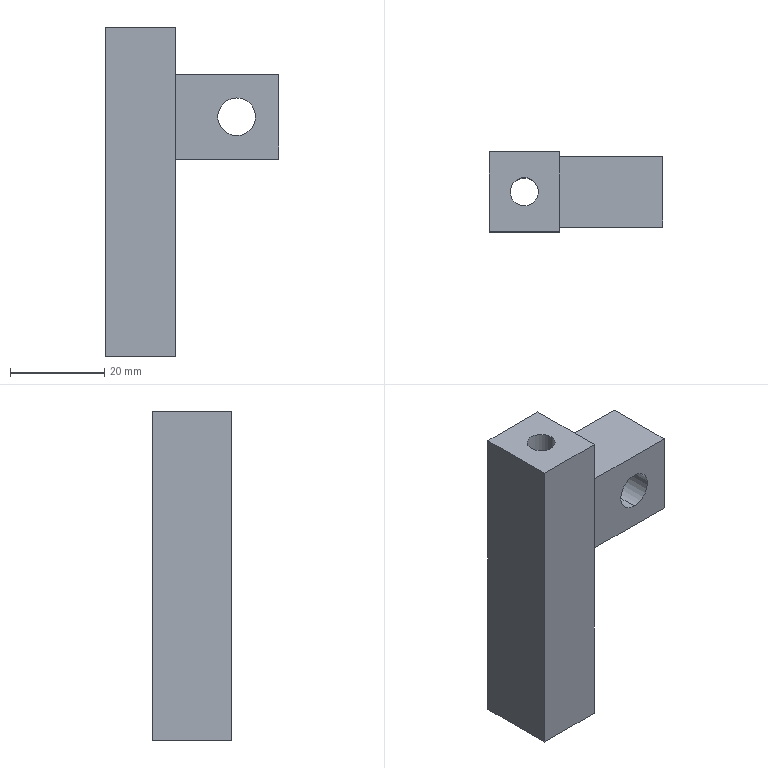Part | SolidWorks | features Cut 2, Extrusion 1, ICE 1 | 1 solid | 15 faces | box 37 x 17 x 70 mm | volume 21057 mm3 | plane 11 | cylinder 4 | commonest cylinder face diameters 6 x2 8 x2
STEP:
#1=CARTESIAN_POINT('',(-11.,-8.806,5.));
#2=VERTEX_POINT('',#1);
#3=CARTESIAN_POINT('',(-11.,-8.806,13.));
#4=VERTEX_POINT('',#3);
#5=CARTESIAN_POINT('',(-11.,-8.806,9.));
#6=DIRECTION('',(0.,1.,0.));
#7=DIRECTION('',(-1.,0.,0.));
#8=AXIS2_PLACEMENT_3D('',#5,#6,#7);
#9=CIRCLE('',#8,4.);
#10=EDGE_CURVE('',#2,#4,#9,.T.);
#11=ORIENTED_EDGE('',*,*,#10,.F.);
#12=CARTESIAN_POINT('',(-11.,6.194,5.));
#13=VERTEX_POINT('',#12);
#14=CARTESIAN_POINT('',(-11.,-34.806,5.));
#15=DIRECTION('',(0.,1.,0.));
#16=VECTOR('',#15,1000.);
#17=LINE('',#14,#16);
#18=EDGE_CURVE('',#2,#13,#17,.T.);
#19=ORIENTED_EDGE('',*,*,#18,.T.);
#20=CARTESIAN_POINT('',(-11.,6.194,13.));
#21=VERTEX_POINT('',#20);
#22=CARTESIAN_POINT('',(-11.,6.194,9.));
#23=DIRECTION('',(0.,1.,0.));
#24=DIRECTION('',(0.,0.,1.));
#25=AXIS2_PLACEMENT_3D('',#22,#23,#24);
#26=CIRCLE('',#25,4.);
#27=EDGE_CURVE('',#13,#21,#26,.T.);
#28=ORIENTED_EDGE('',*,*,#27,.T.);
#29=CARTESIAN_POINT('',(-11.,-34.806,13.));
#30=DIRECTION('',(0.,1.,0.));
#31=VECTOR('',#30,1000.);
#32=LINE('',#29,#31);
#33=EDGE_CURVE('',#4,#21,#32,.T.);
#34=ORIENTED_EDGE('',*,*,#33,.F.);
#35=EDGE_LOOP('',(#11,#19,#28,#34));
#36=FACE_OUTER_BOUND('',#35,.T.);
#37=CARTESIAN_POINT('',(-11.,-34.806,9.));
#38=DIRECTION('',(0.,1.,0.));
#39=DIRECTION('',(0.,0.,1.));
#40=AXIS2_PLACEMENT_3D('',#37,#38,#39);
#41=CYLINDRICAL_SURFACE('',#40,4.);
#42=ADVANCED_FACE('',(#36),#41,.F.);
#43=CARTESIAN_POINT('',(-34.5,-1.306,-42.));
#44=VERTEX_POINT('',#43);
#45=CARTESIAN_POINT('',(-28.5,-1.306,-42.));
#46=VERTEX_POINT('',#45);
#47=CARTESIAN_POINT('',(-31.5,-1.306,-42.));
#48=DIRECTION('',(0.,0.,1.));
#49=DIRECTION('',(1.,0.,0.));
#50=AXIS2_PLACEMENT_3D('',#47,#48,#49);
#51=CIRCLE('',#50,3.);
#52=EDGE_CURVE('',#44,#46,#51,.T.);
#53=ORIENTED_EDGE('',*,*,#52,.F.);
#54=CARTESIAN_POINT('',(-34.5,-1.306,28.));
#55=VERTEX_POINT('',#54);
#56=CARTESIAN_POINT('',(-34.5,-1.306,-82.));
#57=DIRECTION('',(0.,0.,1.));
#58=VECTOR('',#57,1000.);
#59=LINE('',#56,#58);
#60=EDGE_CURVE('',#44,#55,#59,.T.);
#61=ORIENTED_EDGE('',*,*,#60,.T.);
#62=CARTESIAN_POINT('',(-28.5,-1.306,28.));
#63=VERTEX_POINT('',#62);
#64=CARTESIAN_POINT('',(-31.5,-1.306,28.));
#65=DIRECTION('',(0.,0.,1.));
#66=DIRECTION('',(1.,0.,0.));
#67=AXIS2_PLACEMENT_3D('',#64,#65,#66);
#68=CIRCLE('',#67,3.);
#69=EDGE_CURVE('',#55,#63,#68,.T.);
#70=ORIENTED_EDGE('',*,*,#69,.T.);
#71=CARTESIAN_POINT('',(-28.5,-1.306,-82.));
#72=DIRECTION('',(0.,0.,1.));
#73=VECTOR('',#72,1000.);
#74=LINE('',#71,#73);
#75=EDGE_CURVE('',#46,#63,#74,.T.);
#76=ORIENTED_EDGE('',*,*,#75,.F.);
#77=EDGE_LOOP('',(#53,#61,#70,#76));
#78=FACE_OUTER_BOUND('',#77,.T.);
#79=CARTESIAN_POINT('',(-31.5,-1.306,-82.));
#80=DIRECTION('',(0.,0.,1.));
#81=DIRECTION('',(1.,0.,0.));
#82=AXIS2_PLACEMENT_3D('',#79,#80,#81);
#83=CYLINDRICAL_SURFACE('',#82,3.);
#84=ADVANCED_FACE('',(#78),#83,.F.);
#85=CARTESIAN_POINT('',(-2.,-8.806,0.));
#86=VERTEX_POINT('',#85);
#87=CARTESIAN_POINT('',(-2.,6.194,0.));
#88=VERTEX_POINT('',#87);
#89=CARTESIAN_POINT('',(-2.,-8.806,0.));
#90=DIRECTION('',(0.,1.,0.));
#91=VECTOR('',#90,1000.);
#92=LINE('',#89,#91);
#93=EDGE_CURVE('',#86,#88,#92,.T.);
#94=ORIENTED_EDGE('',*,*,#93,.T.);
#95=CARTESIAN_POINT('',(-2.,6.194,18.));
#96=VERTEX_POINT('',#95);
#97=CARTESIAN_POINT('',(-2.,6.194,18.));
#98=DIRECTION('',(0.,0.,-1.));
#99=VECTOR('',#98,1000.);
#100=LINE('',#97,#99);
#101=EDGE_CURVE('',#96,#88,#100,.T.);
#102=ORIENTED_EDGE('',*,*,#101,.F.);
#103=CARTESIAN_POINT('',(-2.,-8.806,18.));
#104=VERTEX_POINT('',#103);
#105=CARTESIAN_POINT('',(-2.,-8.806,18.));
#106=DIRECTION('',(0.,1.,0.));
#107=VECTOR('',#106,1000.);
#108=LINE('',#105,#107);
#109=EDGE_CURVE('',#104,#96,#108,.T.);
#110=ORIENTED_EDGE('',*,*,#109,.F.);
#111=CARTESIAN_POINT('',(-2.,-8.806,18.));
#112=DIRECTION('',(0.,0.,-1.));
#113=VECTOR('',#112,1000.);
#114=LINE('',#111,#113);
#115=EDGE_CURVE('',#104,#86,#114,.T.);
#116=ORIENTED_EDGE('',*,*,#115,.T.);
#117=EDGE_LOOP('',(#94,#102,#110,#116));
#118=FACE_OUTER_BOUND('',#117,.T.);
#119=CARTESIAN_POINT('',(-2.,-8.806,18.));
#120=DIRECTION('',(-1.,0.,0.));
#121=DIRECTION('',(0.,0.,1.));
#122=AXIS2_PLACEMENT_3D('',#119,#120,#121);
#123=PLANE('',#122);
#124=ADVANCED_FACE('',(#118),#123,.F.);
#125=CARTESIAN_POINT('',(-11.,6.194,9.));
#126=DIRECTION('',(0.,1.,0.));
#127=DIRECTION('',(0.,0.,1.));
#128=AXIS2_PLACEMENT_3D('',#125,#126,#127);
#129=CIRCLE('',#128,4.);
#130=EDGE_CURVE('',#21,#13,#129,.T.);
#131=ORIENTED_EDGE('',*,*,#130,.F.);
#132=ORIENTED_EDGE('',*,*,#27,.F.);
#133=EDGE_LOOP('',(#131,#132));
#134=FACE_BOUND('',#133,.T.);
#135=CARTESIAN_POINT('',(-24.,6.194,0.));
#136=VERTEX_POINT('',#135);
#137=CARTESIAN_POINT('',(-2.,6.194,0.));
#138=DIRECTION('',(-1.,0.,0.));
#139=VECTOR('',#138,1000.);
#140=LINE('',#137,#139);
#141=EDGE_CURVE('',#88,#136,#140,.T.);
#142=ORIENTED_EDGE('',*,*,#141,.T.);
#143=CARTESIAN_POINT('',(-24.,6.194,18.));
#144=VERTEX_POINT('',#143);
#145=CARTESIAN_POINT('',(-24.,6.194,18.));
#146=DIRECTION('',(0.,0.,-1.));
#147=VECTOR('',#146,1000.);
#148=LINE('',#145,#147);
#149=EDGE_CURVE('',#144,#136,#148,.T.);
#150=ORIENTED_EDGE('',*,*,#149,.F.);
#151=CARTESIAN_POINT('',(-2.,6.194,18.));
#152=DIRECTION('',(-1.,0.,0.));
#153=VECTOR('',#152,1000.);
#154=LINE('',#151,#153);
#155=EDGE_CURVE('',#96,#144,#154,.T.);
#156=ORIENTED_EDGE('',*,*,#155,.F.);
#157=ORIENTED_EDGE('',*,*,#101,.T.);
#158=EDGE_LOOP('',(#142,#150,#156,#157));
#159=FACE_OUTER_BOUND('',#158,.T.);
#160=CARTESIAN_POINT('',(-2.,6.194,18.));
#161=DIRECTION('',(0.,-1.,0.));
#162=DIRECTION('',(1.,0.,0.));
#163=AXIS2_PLACEMENT_3D('',#160,#161,#162);
#164=PLANE('',#163);
#165=ADVANCED_FACE('',(#134,#159),#164,.F.);
#166=CARTESIAN_POINT('',(-11.,-8.806,9.));
#167=DIRECTION('',(0.,1.,0.));
#168=DIRECTION('',(-1.,0.,0.));
#169=AXIS2_PLACEMENT_3D('',#166,#167,#168);
#170=CIRCLE('',#169,4.);
#171=EDGE_CURVE('',#4,#2,#170,.T.);
#172=ORIENTED_EDGE('',*,*,#171,.T.);
#173=ORIENTED_EDGE('',*,*,#10,.T.);
#174=EDGE_LOOP('',(#172,#173));
#175=FACE_BOUND('',#174,.T.);
#176=CARTESIAN_POINT('',(-24.,-8.806,0.));
#177=VERTEX_POINT('',#176);
#178=CARTESIAN_POINT('',(-2.,-8.806,0.));
#179=DIRECTION('',(1.,0.,0.));
#180=VECTOR('',#179,1000.);
#181=LINE('',#178,#180);
#182=EDGE_CURVE('',#177,#86,#181,.T.);
#183=ORIENTED_EDGE('',*,*,#182,.T.);
#184=ORIENTED_EDGE('',*,*,#115,.F.);
#185=CARTESIAN_POINT('',(-24.,-8.806,18.));
#186=VERTEX_POINT('',#185);
#187=CARTESIAN_POINT('',(-2.,-8.806,18.));
#188=DIRECTION('',(1.,0.,0.));
#189=VECTOR('',#188,1000.);
#190=LINE('',#187,#189);
#191=EDGE_CURVE('',#186,#104,#190,.T.);
#192=ORIENTED_EDGE('',*,*,#191,.F.);
#193=CARTESIAN_POINT('',(-24.,-8.806,18.));
#194=DIRECTION('',(0.,0.,-1.));
#195=VECTOR('',#194,1000.);
#196=LINE('',#193,#195);
#197=EDGE_CURVE('',#186,#177,#196,.T.);
#198=ORIENTED_EDGE('',*,*,#197,.T.);
#199=EDGE_LOOP('',(#183,#184,#192,#198));
#200=FACE_OUTER_BOUND('',#199,.T.);
#201=CARTESIAN_POINT('',(-2.,-8.806,18.));
#202=DIRECTION('',(0.,1.,0.));
#203=DIRECTION('',(-1.,0.,0.));
#204=AXIS2_PLACEMENT_3D('',#201,#202,#203);
#205=PLANE('',#204);
#206=ADVANCED_FACE('',(#175,#200),#205,.F.);
#207=ORIENTED_EDGE('',*,*,#109,.T.);
#208=ORIENTED_EDGE('',*,*,#155,.T.);
#209=CARTESIAN_POINT('',(-24.,-8.806,18.));
#210=DIRECTION('',(0.,-1.,0.));
#211=VECTOR('',#210,1000.);
#212=LINE('',#209,#211);
#213=EDGE_CURVE('',#144,#186,#212,.T.);
#214=ORIENTED_EDGE('',*,*,#213,.T.);
#215=ORIENTED_EDGE('',*,*,#191,.T.);
#216=EDGE_LOOP('',(#207,#208,#214,#215));
#217=FACE_OUTER_BOUND('',#216,.T.);
#218=CARTESIAN_POINT('',(0.,0.,18.));
#219=DIRECTION('',(0.,0.,1.));
#220=DIRECTION('',(1.,0.,0.));
#221=AXIS2_PLACEMENT_3D('',#218,#219,#220);
#222=PLANE('',#221);
#223=ADVANCED_FACE('',(#217),#222,.T.);
#224=ORIENTED_EDGE('',*,*,#93,.F.);
#225=ORIENTED_EDGE('',*,*,#182,.F.);
#226=CARTESIAN_POINT('',(-24.,-8.806,0.));
#227=DIRECTION('',(0.,-1.,0.));
#228=VECTOR('',#227,1000.);
#229=LINE('',#226,#228);
#230=EDGE_CURVE('',#136,#177,#229,.T.);
#231=ORIENTED_EDGE('',*,*,#230,.F.);
#232=ORIENTED_EDGE('',*,*,#141,.F.);
#233=EDGE_LOOP('',(#224,#225,#231,#232));
#234=FACE_OUTER_BOUND('',#233,.T.);
#235=CARTESIAN_POINT('',(0.,0.,0.));
#236=DIRECTION('',(0.,0.,1.));
#237=DIRECTION('',(1.,0.,0.));
#238=AXIS2_PLACEMENT_3D('',#235,#236,#237);
#239=PLANE('',#238);
#240=ADVANCED_FACE('',(#234),#239,.F.);
#241=CARTESIAN_POINT('',(-24.,-9.806,28.));
#242=VERTEX_POINT('',#241);
#243=CARTESIAN_POINT('',(-24.,7.194,28.));
#244=VERTEX_POINT('',#243);
#245=CARTESIAN_POINT('',(-24.,7.194,28.));
#246=DIRECTION('',(0.,1.,0.));
#247=VECTOR('',#246,1000.);
#248=LINE('',#245,#247);
#249=EDGE_CURVE('',#242,#244,#248,.T.);
#250=ORIENTED_EDGE('',*,*,#249,.F.);
#251=CARTESIAN_POINT('',(-24.,-9.806,-42.));
#252=VERTEX_POINT('',#251);
#253=CARTESIAN_POINT('',(-24.,-9.806,-42.));
#254=DIRECTION('',(0.,0.,1.));
#255=VECTOR('',#254,1000.);
#256=LINE('',#253,#255);
#257=EDGE_CURVE('',#252,#242,#256,.T.);
#258=ORIENTED_EDGE('',*,*,#257,.F.);
#259=CARTESIAN_POINT('',(-24.,7.194,-42.));
#260=VERTEX_POINT('',#259);
#261=CARTESIAN_POINT('',(-24.,7.194,-42.));
#262=DIRECTION('',(0.,-1.,0.));
#263=VECTOR('',#262,1000.);
#264=LINE('',#261,#263);
#265=EDGE_CURVE('',#260,#252,#264,.T.);
#266=ORIENTED_EDGE('',*,*,#265,.F.);
#267=CARTESIAN_POINT('',(-24.,7.194,-42.));
#268=DIRECTION('',(0.,0.,-1.));
#269=VECTOR('',#268,1000.);
#270=LINE('',#267,#269);
#271=EDGE_CURVE('',#244,#260,#270,.T.);
#272=ORIENTED_EDGE('',*,*,#271,.F.);
#273=EDGE_LOOP('',(#250,#258,#266,#272));
#274=FACE_OUTER_BOUND('',#273,.T.);
#275=ORIENTED_EDGE('',*,*,#149,.T.);
#276=ORIENTED_EDGE('',*,*,#230,.T.);
#277=ORIENTED_EDGE('',*,*,#197,.F.);
#278=ORIENTED_EDGE('',*,*,#213,.F.);
#279=EDGE_LOOP('',(#275,#276,#277,#278));
#280=FACE_BOUND('',#279,.T.);
#281=CARTESIAN_POINT('',(-24.,0.,0.));
#282=DIRECTION('',(-1.,0.,0.));
#283=DIRECTION('',(0.,0.,1.));
#284=AXIS2_PLACEMENT_3D('',#281,#282,#283);
#285=PLANE('',#284);
#286=ADVANCED_FACE('',(#274,#280),#285,.F.);
#287=CARTESIAN_POINT('',(-31.5,-1.306,28.));
#288=DIRECTION('',(0.,0.,1.));
#289=DIRECTION('',(1.,0.,0.));
#290=AXIS2_PLACEMENT_3D('',#287,#288,#289);
#291=CIRCLE('',#290,3.);
#292=EDGE_CURVE('',#63,#55,#291,.T.);
#293=ORIENTED_EDGE('',*,*,#292,.F.);
#294=ORIENTED_EDGE('',*,*,#69,.F.);
#295=EDGE_LOOP('',(#293,#294));
#296=FACE_BOUND('',#295,.T.);
#297=ORIENTED_EDGE('',*,*,#249,.T.);
#298=CARTESIAN_POINT('',(-39.,7.194,28.));
#299=VERTEX_POINT('',#298);
#300=CARTESIAN_POINT('',(-39.,7.194,28.));
#301=DIRECTION('',(1.,0.,0.));
#302=VECTOR('',#301,1000.);
#303=LINE('',#300,#302);
#304=EDGE_CURVE('',#299,#244,#303,.T.);
#305=ORIENTED_EDGE('',*,*,#304,.F.);
#306=CARTESIAN_POINT('',(-39.,-9.806,28.));
#307=VERTEX_POINT('',#306);
#308=CARTESIAN_POINT('',(-39.,7.194,28.));
#309=DIRECTION('',(0.,1.,0.));
#310=VECTOR('',#309,1000.);
#311=LINE('',#308,#310);
#312=EDGE_CURVE('',#307,#299,#311,.T.);
#313=ORIENTED_EDGE('',*,*,#312,.F.);
#314=CARTESIAN_POINT('',(-39.,-9.806,28.));
#315=DIRECTION('',(1.,0.,0.));
#316=VECTOR('',#315,1000.);
#317=LINE('',#314,#316);
#318=EDGE_CURVE('',#307,#242,#317,.T.);
#319=ORIENTED_EDGE('',*,*,#318,.T.);
#320=EDGE_LOOP('',(#297,#305,#313,#319));
#321=FACE_OUTER_BOUND('',#320,.T.);
#322=CARTESIAN_POINT('',(-39.,7.194,28.));
#323=DIRECTION('',(0.,0.,-1.));
#324=DIRECTION('',(0.,1.,0.));
#325=AXIS2_PLACEMENT_3D('',#322,#323,#324);
#326=PLANE('',#325);
#327=ADVANCED_FACE('',(#296,#321),#326,.F.);
#328=ORIENTED_EDGE('',*,*,#271,.T.);
#329=CARTESIAN_POINT('',(-39.,7.194,-42.));
#330=VERTEX_POINT('',#329);
#331=CARTESIAN_POINT('',(-39.,7.194,-42.));
#332=DIRECTION('',(1.,0.,0.));
#333=VECTOR('',#332,1000.);
#334=LINE('',#331,#333);
#335=EDGE_CURVE('',#330,#260,#334,.T.);
#336=ORIENTED_EDGE('',*,*,#335,.F.);
#337=CARTESIAN_POINT('',(-39.,7.194,-42.));
#338=DIRECTION('',(0.,0.,-1.));
#339=VECTOR('',#338,1000.);
#340=LINE('',#337,#339);
#341=EDGE_CURVE('',#299,#330,#340,.T.);
#342=ORIENTED_EDGE('',*,*,#341,.F.);
#343=ORIENTED_EDGE('',*,*,#304,.T.);
#344=EDGE_LOOP('',(#328,#336,#342,#343));
#345=FACE_OUTER_BOUND('',#344,.T.);
#346=CARTESIAN_POINT('',(-39.,7.194,-42.));
#347=DIRECTION('',(0.,-1.,0.));
#348=DIRECTION('',(0.,0.,-1.));
#349=AXIS2_PLACEMENT_3D('',#346,#347,#348);
#350=PLANE('',#349);
#351=ADVANCED_FACE('',(#345),#350,.F.);
#352=CARTESIAN_POINT('',(-31.5,-1.306,-42.));
#353=DIRECTION('',(0.,0.,1.));
#354=DIRECTION('',(1.,0.,0.));
#355=AXIS2_PLACEMENT_3D('',#352,#353,#354);
#356=CIRCLE('',#355,3.);
#357=EDGE_CURVE('',#46,#44,#356,.T.);
#358=ORIENTED_EDGE('',*,*,#357,.T.);
#359=ORIENTED_EDGE('',*,*,#52,.T.);
#360=EDGE_LOOP('',(#358,#359));
#361=FACE_BOUND('',#360,.T.);
#362=ORIENTED_EDGE('',*,*,#265,.T.);
#363=CARTESIAN_POINT('',(-39.,-9.806,-42.));
#364=VERTEX_POINT('',#363);
#365=CARTESIAN_POINT('',(-39.,-9.806,-42.));
#366=DIRECTION('',(1.,0.,0.));
#367=VECTOR('',#366,1000.);
#368=LINE('',#365,#367);
#369=EDGE_CURVE('',#364,#252,#368,.T.);
#370=ORIENTED_EDGE('',*,*,#369,.F.);
#371=CARTESIAN_POINT('',(-39.,7.194,-42.));
#372=DIRECTION('',(0.,-1.,0.));
#373=VECTOR('',#372,1000.);
#374=LINE('',#371,#373);
#375=EDGE_CURVE('',#330,#364,#374,.T.);
#376=ORIENTED_EDGE('',*,*,#375,.F.);
#377=ORIENTED_EDGE('',*,*,#335,.T.);
#378=EDGE_LOOP('',(#362,#370,#376,#377));
#379=FACE_OUTER_BOUND('',#378,.T.);
#380=CARTESIAN_POINT('',(-39.,7.194,-42.));
#381=DIRECTION('',(0.,0.,1.));
#382=DIRECTION('',(1.,0.,0.));
#383=AXIS2_PLACEMENT_3D('',#380,#381,#382);
#384=PLANE('',#383);
#385=ADVANCED_FACE('',(#361,#379),#384,.F.);
#386=ORIENTED_EDGE('',*,*,#257,.T.);
#387=ORIENTED_EDGE('',*,*,#318,.F.);
#388=CARTESIAN_POINT('',(-39.,-9.806,-42.));
#389=DIRECTION('',(0.,0.,1.));
#390=VECTOR('',#389,1000.);
#391=LINE('',#388,#390);
#392=EDGE_CURVE('',#364,#307,#391,.T.);
#393=ORIENTED_EDGE('',*,*,#392,.F.);
#394=ORIENTED_EDGE('',*,*,#369,.T.);
#395=EDGE_LOOP('',(#386,#387,#393,#394));
#396=FACE_OUTER_BOUND('',#395,.T.);
#397=CARTESIAN_POINT('',(-39.,-9.806,-42.));
#398=DIRECTION('',(0.,1.,0.));
#399=DIRECTION('',(0.,0.,1.));
#400=AXIS2_PLACEMENT_3D('',#397,#398,#399);
#401=PLANE('',#400);
#402=ADVANCED_FACE('',(#396),#401,.F.);
#403=ORIENTED_EDGE('',*,*,#312,.T.);
#404=ORIENTED_EDGE('',*,*,#341,.T.);
#405=ORIENTED_EDGE('',*,*,#375,.T.);
#406=ORIENTED_EDGE('',*,*,#392,.T.);
#407=EDGE_LOOP('',(#403,#404,#405,#406));
#408=FACE_OUTER_BOUND('',#407,.T.);
#409=CARTESIAN_POINT('',(-39.,0.,0.));
#410=DIRECTION('',(-1.,0.,0.));
#411=DIRECTION('',(0.,0.,1.));
#412=AXIS2_PLACEMENT_3D('',#409,#410,#411);
#413=PLANE('',#412);
#414=ADVANCED_FACE('',(#408),#413,.T.);
#415=ORIENTED_EDGE('',*,*,#60,.F.);
#416=ORIENTED_EDGE('',*,*,#357,.F.);
#417=ORIENTED_EDGE('',*,*,#75,.T.);
#418=ORIENTED_EDGE('',*,*,#292,.T.);
#419=EDGE_LOOP('',(#415,#416,#417,#418));
#420=FACE_OUTER_BOUND('',#419,.T.);
#421=CARTESIAN_POINT('',(-31.5,-1.306,-82.));
#422=DIRECTION('',(0.,0.,1.));
#423=DIRECTION('',(1.,0.,0.));
#424=AXIS2_PLACEMENT_3D('',#421,#422,#423);
#425=CYLINDRICAL_SURFACE('',#424,3.);
#426=ADVANCED_FACE('',(#420),#425,.F.);
#427=ORIENTED_EDGE('',*,*,#18,.F.);
#428=ORIENTED_EDGE('',*,*,#171,.F.);
#429=ORIENTED_EDGE('',*,*,#33,.T.);
#430=ORIENTED_EDGE('',*,*,#130,.T.);
#431=EDGE_LOOP('',(#427,#428,#429,#430));
#432=FACE_OUTER_BOUND('',#431,.T.);
#433=CARTESIAN_POINT('',(-11.,-34.806,9.));
#434=DIRECTION('',(0.,1.,0.));
#435=DIRECTION('',(0.,0.,1.));
#436=AXIS2_PLACEMENT_3D('',#433,#434,#435);
#437=CYLINDRICAL_SURFACE('',#436,4.);
#438=ADVANCED_FACE('',(#432),#437,.F.);
#439=CLOSED_SHELL('',(#42,#84,#124,#165,#206,#223,#240,#286,#327,#351,#385,#402,#414,#426,#438));
#440=MANIFOLD_SOLID_BREP('',#439);
#441=CARTESIAN_POINT('',(0.,0.,0.));
#442=DIRECTION('',(0.,0.,1.));
#443=DIRECTION('',(1.,0.,0.));
#444=AXIS2_PLACEMENT_3D('',#441,#442,#443);
#445=(LENGTH_UNIT()NAMED_UNIT(*)SI_UNIT(.MILLI.,.METRE.));
#446=UNCERTAINTY_MEASURE_WITH_UNIT(LENGTH_MEASURE(0.00001),#445,'','');
#447=(NAMED_UNIT(*)PLANE_ANGLE_UNIT()SI_UNIT($,.RADIAN.));
#448=(NAMED_UNIT(*)SI_UNIT($,.STERADIAN.)SOLID_ANGLE_UNIT());
#449=(GEOMETRIC_REPRESENTATION_CONTEXT(3)GLOBAL_UNCERTAINTY_ASSIGNED_CONTEXT((#446))GLOBAL_UNIT_ASSIGNED_CONTEXT((#445,#447,#448))REPRESENTATION_CONTEXT('',''));
#450=ADVANCED_BREP_SHAPE_REPRESENTATION('',(#440,#444),#449);